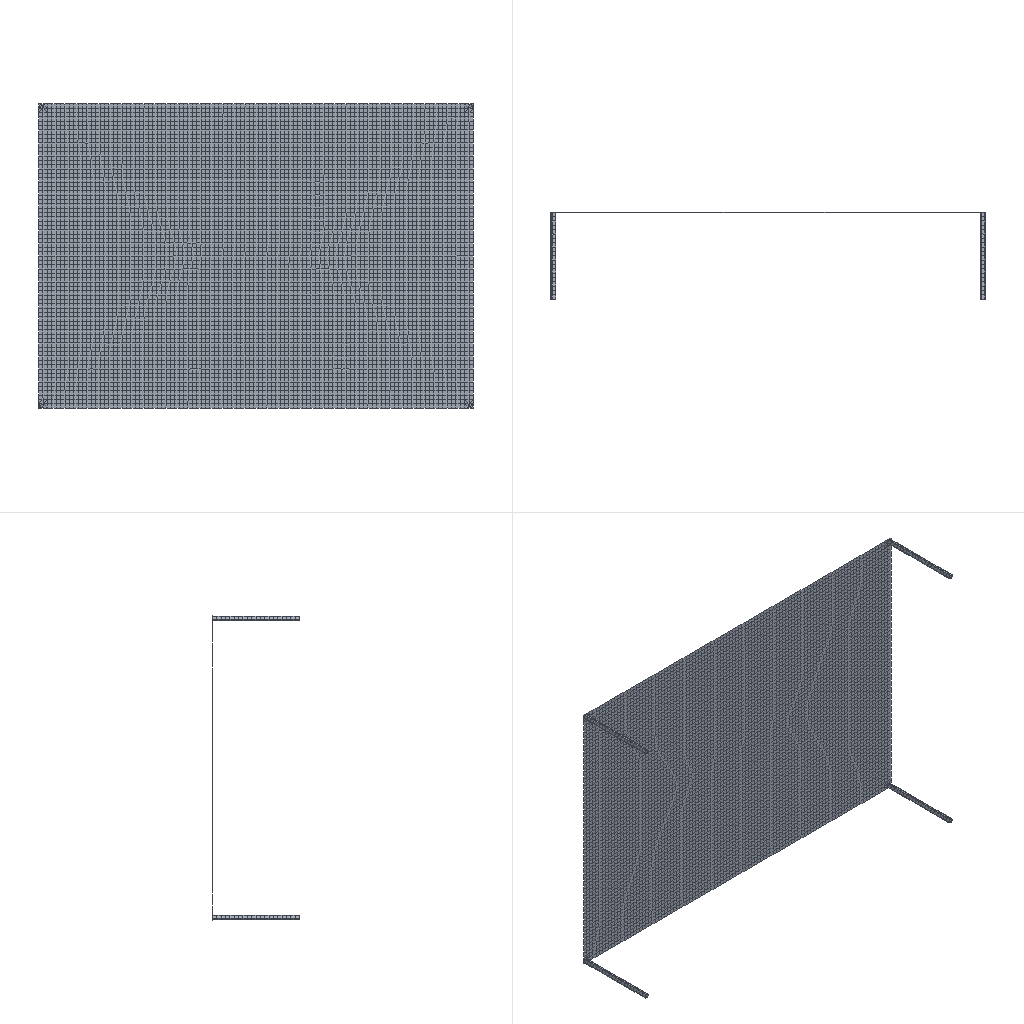Simulation study | ansys workbench
Set-up summary:
category,name,step,type,value,unit,region
solver,ansys_workbench
units,mm-N-s-tonne (MPa),,stated,"/units,MPA"
analysis,LS1,,modal,method=lanb; n_modes=6
load_step,LS1,LS1,modal
mesh,nodes,,,9420
mesh,elements,,,7314
element_type,SHELL181,,,6930
element_type,SOLID186,,,320
element_type,TARGE170,,,32
element_type,CONTA174,,,32
material,Structural Steel,,E,200000,tonne s^-2 mm^-1
material,Structural Steel,,nu,0.3
material,Structural Steel,,density,7.85e-09,tonne mm^-3
material,Structural Steel,,conductivity,60.5,tonne mm s^-3 C^-1
material,Structural Steel,,specific_heat,4.34e+08,mm^2 s^-2 C^-1
material,Structural Steel,,cte,1.2e-05,C^-1
material,Structural Steel,,permeability,10000
material,Structural Steel,,resistivity,0.00017,ohm mm
contact,Contact Region,,bonded (always),element=CONTA174
contact,Contact Region 2,,bonded (always),element=CONTA174
contact,Contact Region 3,,bonded (always),element=CONTA174
contact,Contact Region 4,,bonded (always),element=CONTA174
Ansys APDL input file, long lists of numbers shortened:
/batch
/config,noeldb,1     ! force off writing results to database
*get,_wallstrt,active,,time,wall
! ANSYS input file written by Workbench version 2021 R1
! File used for geometry attach:
/title,________--__ (J5)
! ****** Begin Custom Load Command Snippet ******
/COM, ACT Extensions:
/COM,     LSDYNA, 2021.1
/COM,
! ****** End   Custom Load Command Snippet ******
*DIM,_wb_ProjectScratch_dir,string,248
_wb_ProjectScratch_dir(1) = ''
*DIM,_wb_SolverFiles_dir,string,248
_wb_SolverFiles_dir(1) = ''
*DIM,_wb_userfiles_dir,string,248
_wb_userfiles_dir(1) = ''
/com,--- Data in consistent NMM units. See Solving Units in the help system for more information.
/units,MPA
/nopr
/wb,file,start              !  signify a WB generated input file
/prep7
! Turn off shape checking because checks already performed inside WB mesher.
! See help system for more information.
SHPP,OFF,,NOWARN
/nolist
etcon,set             ! allow ANSYS to choose best KEYOP's for 180x elements, resets any applicable keyopt to MAPDL defaults
/com,*********** Nodes for the whole assembly ***********
nblock,3,,10362
(1i9,3e20.9e3)
     8261     2.493292603E+03     0.000000000E+00    -1.710919547E+03
! (9419 more lines like these left out)
-1
/wb,elem,start            !  set before creation of elements
/com,*********** Elements for Body 1 "______-______|NONE" ***********
et,1,181
keyo,1,3,2
eblock,19,solid,,6930
(19i9)
        1        1        1        1        0        0        0        0        4        0      321      339      401      400      340
! (6929 more lines like these left out)
-1
/com,*********** Elements for Body 2 "______-____|____-____1" ***********
et,2,186
keyo,2,2,1          ! set full integration on SOLID186
eblock,19,solid,,80
(19i9)
        2        2        2        2        0        0        0        0       20        0        1     7129     7268     7188     7190     7168     7267     7187     7209
! (159 more lines like these left out)
-1
/com,*********** Elements for Body 3 "______-____|____-____1[2]" ***********
et,3,186
keyo,3,2,1          ! set full integration on SOLID186
eblock,19,solid,,80
(19i9)
        3        3        3        3        0        0        0        0       20        0       81     7709     7848     7768     7770     7748     7847     7767     7789
! (159 more lines like these left out)
-1
/com,*********** Elements for Body 4 "______-____|____-____1[3]" ***********
et,4,186
keyo,4,2,1          ! set full integration on SOLID186
eblock,19,solid,,80
(19i9)
        4        4        4        4        0        0        0        0       20        0      161     8289     8428     8348     8350     8328     8427     8347     8369
! (159 more lines like these left out)
-1
/com,*********** Elements for Body 5 "______-____|____-____1[4]" ***********
et,5,186
keyo,5,2,1          ! set full integration on SOLID186
eblock,19,solid,,80
(19i9)
        5        5        5        5        0        0        0        0       20        0      241     8869     9008     8928     8930     8908     9007     8927     8949
! (159 more lines like these left out)
-1
/wb,elem,end               !  done creating elements
/com,*********** Send User Defined Coordinate System(s) ***********
csys,0
toffst,273.15,  ! Temperature offset from absolute zero
/com,*********** Set Reference Temperature ***********
tref,22.
/wb,mat,start              !  starting to send materials
/com,*********** Send Materials ***********
Temperature = 'TEMP' ! Temperature
MP,DENS,1,7.85e-09,	! tonne mm^-3
MP,ALPX,1,1.2e-05,	! C^-1
MP,C,1,434000000,	! mm^2 s^-2 C^-1
MP,KXX,1,60.5,	! tonne mm s^-3 C^-1
MP,RSVX,1,0.00017,	! ohm mm
MP,EX,1,200000,	! tonne s^-2 mm^-1
MP,NUXY,1,0.3,
MP,MURX,1,10000,
Temperature = 'TEMP' ! Temperature
MP,DENS,2,7.85e-09,	! tonne mm^-3
MP,ALPX,2,1.2e-05,	! C^-1
MP,C,2,434000000,	! mm^2 s^-2 C^-1
MP,KXX,2,60.5,	! tonne mm s^-3 C^-1
MP,RSVX,2,0.00017,	! ohm mm
MP,EX,2,200000,	! tonne s^-2 mm^-1
MP,NUXY,2,0.3,
MP,MURX,2,10000,
Temperature = 'TEMP' ! Temperature
MP,DENS,3,7.85e-09,	! tonne mm^-3
MP,ALPX,3,1.2e-05,	! C^-1
MP,C,3,434000000,	! mm^2 s^-2 C^-1
MP,KXX,3,60.5,	! tonne mm s^-3 C^-1
MP,RSVX,3,0.00017,	! ohm mm
MP,EX,3,200000,	! tonne s^-2 mm^-1
MP,NUXY,3,0.3,
MP,MURX,3,10000,
Temperature = 'TEMP' ! Temperature
MP,DENS,4,7.85e-09,	! tonne mm^-3
MP,ALPX,4,1.2e-05,	! C^-1
MP,C,4,434000000,	! mm^2 s^-2 C^-1
MP,KXX,4,60.5,	! tonne mm s^-3 C^-1
MP,RSVX,4,0.00017,	! ohm mm
MP,EX,4,200000,	! tonne s^-2 mm^-1
MP,NUXY,4,0.3,
MP,MURX,4,10000,
Temperature = 'TEMP' ! Temperature
MP,DENS,5,7.85e-09,	! tonne mm^-3
MP,ALPX,5,1.2e-05,	! C^-1
MP,C,5,434000000,	! mm^2 s^-2 C^-1
MP,KXX,5,60.5,	! tonne mm s^-3 C^-1
MP,RSVX,5,0.00017,	! ohm mm
MP,EX,5,200000,	! tonne s^-2 mm^-1
MP,NUXY,5,0.3,
MP,MURX,5,10000,
/wb,mat,end                !  done sending materials
/com,*********** Send Sheet Properties ***********
sectype,1,shell
secdata,85.
secoff,bot
!************************* Model Summary ********************
!______-______|NONE,	结构钢,	matid,	1
!______-____|____-____1,	结构钢,	matid,	2
!______-____|____-____1[2],	结构钢,	matid,	3
!______-____|____-____1[3],	结构钢,	matid,	4
!______-____|____-____1[4],	结构钢,	matid,	5
!************************* End Model Summary ********************
! get the diagonal of the bounding box. Needed later for other things
*get,_xmin,node,,mnloc,x
*get,_ymin,node,,mnloc,y
*get,_zmin,node,,mnloc,z
*get,_xmax,node,,mxloc,x
*get,_ymax,node,,mxloc,y
*get,_zmax,node,,mxloc,z
_ASMDIAG=(_xmax-_xmin)*(_xmax-_xmin)+(_ymax-_ymin)*(_ymax-_ymin)+(_zmax-_zmin)*(_zmax-_zmin)
_ASMDIAG=SQRT(_ASMDIAG)
/wb,contact,start          !  starting to send contact
/com,*********** Create Contact "接触区域" ***********
/com,            Real Constant Set For Above Contact Is 7 & 6
*set,tid,7
*set,cid,6
r,tid
r,cid
et,tid,170
et,cid,174
eblock,10,,,4
(15i9)
     7923        7        7        7        0     4986     4987     4724     4985
     7924        7        7        7        0      241     4986     4985      242
     7925        7        7        7        0      240     4986      241      171
     7926        7        7        7        0      239     4987     4986      240
-1
eblock,10,,,4
(15i9)
     7927        6        6        6        0     4986     4987     4724     4985
     7928        6        6        6        0      241     4986     4985      242
     7929        6        6        6        0      240     4986      241      171
     7930        6        6        6        0      239     4987     4986      240
-1
eblock,10,,,4
(15i9)
     7931        6        7        6        0     7106     7101     7105     7104     7270     7269     7280     7281
     7932        6        7        6        0     7104     7102     7108     7106     7274     7275     7284     7281
     7933        6        7        6        0     7102     7103     7107     7108     7273     7278     7286     7275
     7934        6        7        6        0     7105     7101     7107     7103     7269     7271     7278     7277
-1
eblock,10,,,4
(15i9)
     7935        7        6        7        0     7106     7101     7105     7104     7270     7269     7280     7281
     7936        7        6        7        0     7104     7102     7108     7106     7274     7275     7284     7281
     7937        7        6        7        0     7102     7103     7107     7108     7273     7278     7286     7275
     7938        7        6        7        0     7105     7101     7107     7103     7269     7271     7278     7277
-1
keyo,cid,8,2               ! auto create asymmetric contact (from Program Controlled setting)
keyo,cid,10,0              ! adjust contact stiffness each NR iteration (from Program Controlled setting)
keyo,cid,12,5              ! bonded always
keyo,cid,18,1              ! small sliding turned on by application
keyo,cid,2,0               ! augmented Lagrange (from Program Controlled setting)
keyo,cid,4,0               ! on Gauss point (from Program Controlled setting)
keyo,cid,9,1               ! ignore initial gaps/penetration
keyo,cid,7,0               ! No Prediction
rmod,tid,3,10.      ! FKN
rmod,tid,5,0.       ! ICONT
rmod,tid,6,-15.522  ! PINB
rmod,tid,10,0.      ! CNOF
rmod,tid,12,0.      ! FKT
rmod,tid,36,37      ! WB DSID
rmod,cid,3,10.      ! FKN
rmod,cid,5,0.       ! ICONT
rmod,cid,6,-15.522  ! PINB
rmod,cid,10,0.      ! CNOF
rmod,cid,12,0.      ! FKT
rmod,cid,36,37      ! WB DSID
/com,*********** Create Contact "接触区域 2" ***********
/com,            Real Constant Set For Above Contact Is 9 & 8
*set,tid,9
*set,cid,8
r,tid
r,cid
et,tid,170
et,cid,174
eblock,10,,,4
(15i9)
     7939        9        9        9        0     4889     4890     4723     4888
     7940        9        9        9        0        3     4889     4888        4
     7941        9        9        9        0      338     4889        3        1
     7942        9        9        9        0      337     4890     4889      338
-1
eblock,10,,,4
(15i9)
     7943        8        8        8        0     4889     4890     4723     4888
     7944        8        8        8        0        3     4889     4888        4
     7945        8        8        8        0      338     4889        3        1
     7946        8        8        8        0      337     4890     4889      338
-1
eblock,10,,,4
(15i9)
     7947        8        9        8        0     7686     7681     7685     7684     7850     7849     7860     7861
     7948        8        9        8        0     7684     7682     7688     7686     7854     7855     7864     7861
     7949        8        9        8        0     7682     7683     7687     7688     7853     7858     7866     7855
     7950        8        9        8        0     7685     7681     7687     7683     7849     7851     7858     7857
-1
eblock,10,,,4
(15i9)
     7951        9        8        9        0     7686     7681     7685     7684     7850     7849     7860     7861
     7952        9        8        9        0     7684     7682     7688     7686     7854     7855     7864     7861
     7953        9        8        9        0     7682     7683     7687     7688     7853     7858     7866     7855
     7954        9        8        9        0     7685     7681     7687     7683     7849     7851     7858     7857
-1
keyo,cid,8,2               ! auto create asymmetric contact (from Program Controlled setting)
keyo,cid,10,0              ! adjust contact stiffness each NR iteration (from Program Controlled setting)
keyo,cid,12,5              ! bonded always
keyo,cid,18,1              ! small sliding turned on by application
keyo,cid,2,0               ! augmented Lagrange (from Program Controlled setting)
keyo,cid,4,0               ! on Gauss point (from Program Controlled setting)
keyo,cid,9,1               ! ignore initial gaps/penetration
keyo,cid,7,0               ! No Prediction
rmod,tid,3,10.      ! FKN
rmod,tid,5,0.       ! ICONT
rmod,tid,6,-15.522  ! PINB
rmod,tid,10,0.      ! CNOF
rmod,tid,12,0.      ! FKT
rmod,tid,36,40      ! WB DSID
rmod,cid,3,10.      ! FKN
rmod,cid,5,0.       ! ICONT
rmod,cid,6,-15.522  ! PINB
rmod,cid,10,0.      ! CNOF
rmod,cid,12,0.      ! FKT
rmod,cid,36,40      ! WB DSID
/com,*********** Create Contact "接触区域 3" ***********
/com,            Real Constant Set For Above Contact Is 11 & 10
*set,tid,11
*set,cid,10
r,tid
r,cid
et,tid,170
et,cid,174
eblock,10,,,4
(15i9)
     7955       11       11       11        0     4821     4822     4722     4820
     7956       11       11       11        0       73     4821     4820       74
     7957       11       11       11        0       71     4821       73        2
     7958       11       11       11        0       70     4822     4821       71
-1
eblock,10,,,4
(15i9)
     7959       10       10       10        0     4821     4822     4722     4820
     7960       10       10       10        0       73     4821     4820       74
     7961       10       10       10        0       71     4821       73        2
     7962       10       10       10        0       70     4822     4821       71
-1
eblock,10,,,4
(15i9)
     7963       10       11       10        0     8266     8261     8265     8264     8430     8429     8440     8441
     7964       10       11       10        0     8264     8262     8268     8266     8434     8435     8444     8441
     7965       10       11       10        0     8262     8263     8267     8268     8433     8438     8446     8435
     7966       10       11       10        0     8265     8261     8267     8263     8429     8431     8438     8437
-1
eblock,10,,,4
(15i9)
     7967       11       10       11        0     8266     8261     8265     8264     8430     8429     8440     8441
     7968       11       10       11        0     8264     8262     8268     8266     8434     8435     8444     8441
     7969       11       10       11        0     8262     8263     8267     8268     8433     8438     8446     8435
     7970       11       10       11        0     8265     8261     8267     8263     8429     8431     8438     8437
-1
keyo,cid,8,2               ! auto create asymmetric contact (from Program Controlled setting)
keyo,cid,10,0              ! adjust contact stiffness each NR iteration (from Program Controlled setting)
keyo,cid,12,5              ! bonded always
keyo,cid,18,1              ! small sliding turned on by application
keyo,cid,2,0               ! augmented Lagrange (from Program Controlled setting)
keyo,cid,4,0               ! on Gauss point (from Program Controlled setting)
keyo,cid,9,1               ! ignore initial gaps/penetration
keyo,cid,7,0               ! No Prediction
rmod,tid,3,10.      ! FKN
rmod,tid,5,0.       ! ICONT
rmod,tid,6,-15.522  ! PINB
rmod,tid,10,0.      ! CNOF
rmod,tid,12,0.      ! FKT
rmod,tid,36,43      ! WB DSID
rmod,cid,3,10.      ! FKN
rmod,cid,5,0.       ! ICONT
rmod,cid,6,-15.522  ! PINB
rmod,cid,10,0.      ! CNOF
rmod,cid,12,0.      ! FKT
rmod,cid,36,43      ! WB DSID
/com,*********** Create Contact "接触区域 4" ***********
/com,            Real Constant Set For Above Contact Is 13 & 12
*set,tid,13
*set,cid,12
r,tid
r,cid
et,tid,170
et,cid,174
eblock,10,,,4
(15i9)
     7971       13       13       13        0     5054     4725     4721     5053
     7972       13       13       13        0      169     4725     5054      170
     7973       13       13       13        0      172     5054     5053      173
     7974       13       13       13        0       72      170     5054      172
-1
eblock,10,,,4
(15i9)
     7975       12       12       12        0     5054     4725     4721     5053
     7976       12       12       12        0      169     4725     5054      170
     7977       12       12       12        0      172     5054     5053      173
     7978       12       12       12        0       72      170     5054      172
-1
eblock,10,,,4
(15i9)
     7979       12       13       12        0     8846     8841     8845     8844     9010     9009     9020     9021
     7980       12       13       12        0     8844     8842     8848     8846     9014     9015     9024     9021
     7981       12       13       12        0     8842     8843     8847     8848     9013     9018     9026     9015
     7982       12       13       12        0     8845     8841     8847     8843     9009     9011     9018     9017
-1
eblock,10,,,4
(15i9)
     7983       13       12       13        0     8846     8841     8845     8844     9010     9009     9020     9021
     7984       13       12       13        0     8844     8842     8848     8846     9014     9015     9024     9021
     7985       13       12       13        0     8842     8843     8847     8848     9013     9018     9026     9015
     7986       13       12       13        0     8845     8841     8847     8843     9009     9011     9018     9017
-1
keyo,cid,8,2               ! auto create asymmetric contact (from Program Controlled setting)
keyo,cid,10,0              ! adjust contact stiffness each NR iteration (from Program Controlled setting)
keyo,cid,12,5              ! bonded always
keyo,cid,18,1              ! small sliding turned on by application
keyo,cid,2,0               ! augmented Lagrange (from Program Controlled setting)
keyo,cid,4,0               ! on Gauss point (from Program Controlled setting)
keyo,cid,9,1               ! ignore initial gaps/penetration
keyo,cid,7,0               ! No Prediction
rmod,tid,3,10.      ! FKN
rmod,tid,5,0.       ! ICONT
rmod,tid,6,-15.522  ! PINB
rmod,tid,10,0.      ! CNOF
rmod,tid,12,0.      ! FKT
rmod,tid,36,46      ! WB DSID
rmod,cid,3,10.      ! FKN
rmod,cid,5,0.       ! ICONT
rmod,cid,6,-15.522  ! PINB
rmod,cid,10,0.      ! CNOF
rmod,cid,12,0.      ! FKT
rmod,cid,36,46      ! WB DSID
nsel,all
esel,all
/wb,contact,end            !  done creating contacts
/golist
/wb,load,start             !  starting to send loads
/gst,on,on
fini
*get,_numnode,node,0,count
*get,_numelem,elem,0,count
*get, _MAXELEMNUM, elem, 0, NUM, MAX
*get, _MAXNODENUM, node, 0, NUM, MAX
*get, _MAXELEMTYPE, etyp, 0, NUM, MAX
*get, _MAXREALCONST, real, 0, NUM, MAX
/go
/wb,load,end               !  done creating loads
/com,--- Number of total nodes = %_numnode%
/com,--- Number of contact elements = 64
/com,--- Number of spring elements = 0
/com,--- Number of bearing elements = 0
/com,--- Number of solid elements = 7250
/com,--- Number of condensed parts = 0
/com,--- Number of total elements = %_numelem%
*get,_wallbsol,active,,time,wall
/solu
antype,2                   ! modal analysis
_thickRatio=  0     ! Ratio of thick parts in the model
modopt,lanb,6
outres,erase
outres,all,none
outres,nsol,all
outres,etmp,all
mxpand                    ! default expand in case of complex solution
dmpopt,esav,no
dmpopt,emat,no
dmpopt,full,no
! *********** WB SOLVE COMMAND ***********
! check interactive state
*get,ANSINTER_,active,,int
*if,ANSINTER_,ne,0,then
/eof
*endif
solve
/com *************** Write FE CONNECTORS *********
CEWRITE,file,ce,,INTE
*get,_nmodalsolproc,active,0,numcpu
fini
/nopr
*get,_numnode,node,0,count
*get,_numelem,elem,0,count
*get, _MAXELEMNUM, elem, 0, NUM, MAX
*get, _MAXNODENUM, node, 0, NUM, MAX,,,INTERNAL
*get, _MAXELEMTYPE, etyp, 0, NUM, MAX
*get, _MAXREALCONST, real, 0, NUM, MAX
/gopr
*get,_wallasol,active,,time,wall
/post1
/nopr
*dim,_direction,CHAR,6,1
_direction(1) = 'X'
_direction(2) = 'Y'
_direction(3) = 'Z'
_direction(4) = 'ROTX'
_direction(5) = 'ROTY'
_direction(6) = 'ROTZ'
*get,_lastLS,active,0,set,LSTP
*get,_beginset,active,0,set,nset,first,_lastLS
*get,_endset,active,0,set,nset,last,_lastLS
_nummodes = 0
*if,_endset,gt,0,then
_nummodes = _endset - _beginset + 1
*endif
*do,i_mode,1,_nummodes
   *do,j_component,1,6
			*get,PFACT_%i_mode%_%j_component%,MODE,%i_mode%,PFACT,,DIREC,_direction(%j_component%)
   *enddo
*enddo
*dim,_tmdirection,CHAR,6,1
_tmdirection(1) = 'X'
_tmdirection(2) = 'Y'
_tmdirection(3) = 'Z'
_tmdirection(4) = 'X'
_tmdirection(5) = 'Y'
_tmdirection(6) = 'Z'
*do,j_component,1,6
    *if,j_component,gt,3,then
        *get,TOTALMASS_%j_component%,ELEM,0,IOR,_tmdirection(%j_component%)
    *else
        *get,TOTALMASS_%j_component%,ELEM,0,MTOT,_tmdirection(%j_component%)
    *endif
*enddo
/gopr
xmlo,ENCODING,ISO-8859-1
xmlo,parm
/xml,parm,xml
fini
/gopr
*get,_walldone,active,,time,wall
_preptime=(_wallbsol-_wallstrt)*3600
_solvtime=(_wallasol-_wallbsol)*3600
_posttime=(_walldone-_wallasol)*3600
_totaltim=(_walldone-_wallstrt)*3600
*get,_dlbratio,active,0,solu,dlbr
*get,_combtime,active,0,solu,comb
/com,--- Total number of nodes = %_numnode%
/com,--- Total number of elements = %_numelem%
/com,--- Element load balance ratio = %_dlbratio%
/com,--- Time to combine distributed files = %_combtime%
/wb,file,end               ! done with WB generated input
Results summary:
result,analyses[0].index,,,1
result,analyses[0].system,,,SYS-9
result,analyses[0].deck,,,deck.dat
result,analyses[0].solve_status,,,completed
result,analyses[0].analysis_type,,,modal
result,analyses[0].physics,,,mechanical
result,analyses[0].unit_system,,,"NMM: mm, ton, N, s, mV, mA, degC"
result,analyses[0].n_sets,,,6
result,analyses[0].modal_frequencies_hz[1],,,0
result,analyses[0].modal_frequencies_hz[2],,,0
result,analyses[0].modal_frequencies_hz[3],,,0
result,analyses[0].modal_frequencies_hz[4],,,0.0001636
result,analyses[0].modal_frequencies_hz[5],,,0.0005742
result,analyses[0].modal_frequencies_hz[6],,,0.0008832
result,geometry_export[0][0],,,.step
result,geometry_export[0][1],,,ok
result,geometry_export[0][2],,,5